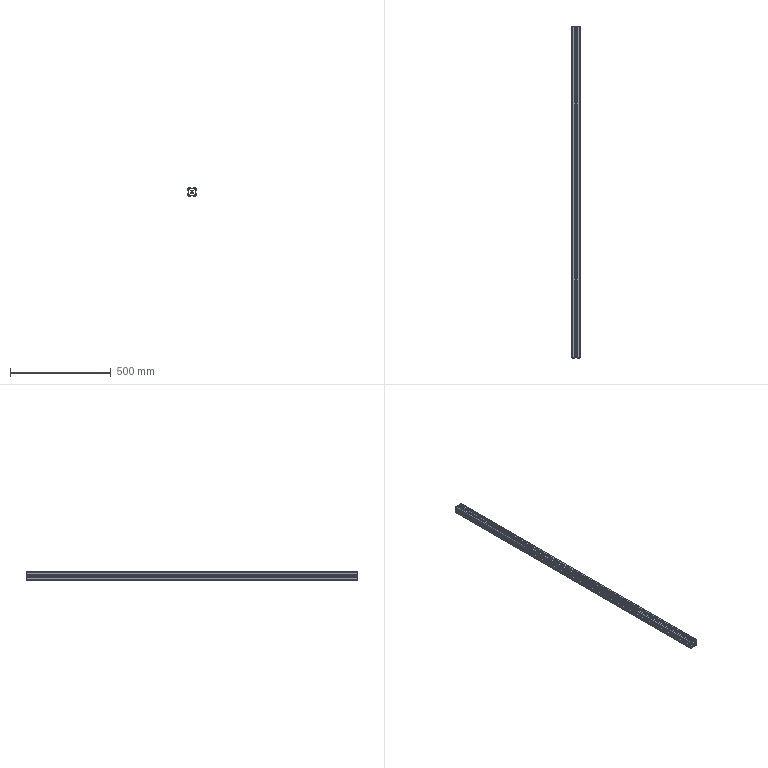Part | SolidWorks | features HoleWzd 1, LPattern 1, WeldMemberFeat 1, WeldmentFeature 1 | 1 solid | 156 faces | box 40 x 1650 x 40 mm | volume 782541 mm3 | plane 118 | cylinder 38 | commonest cylinder face diameters 6.6 x16 11 x12 5 x4 9 x4 6.8 x2